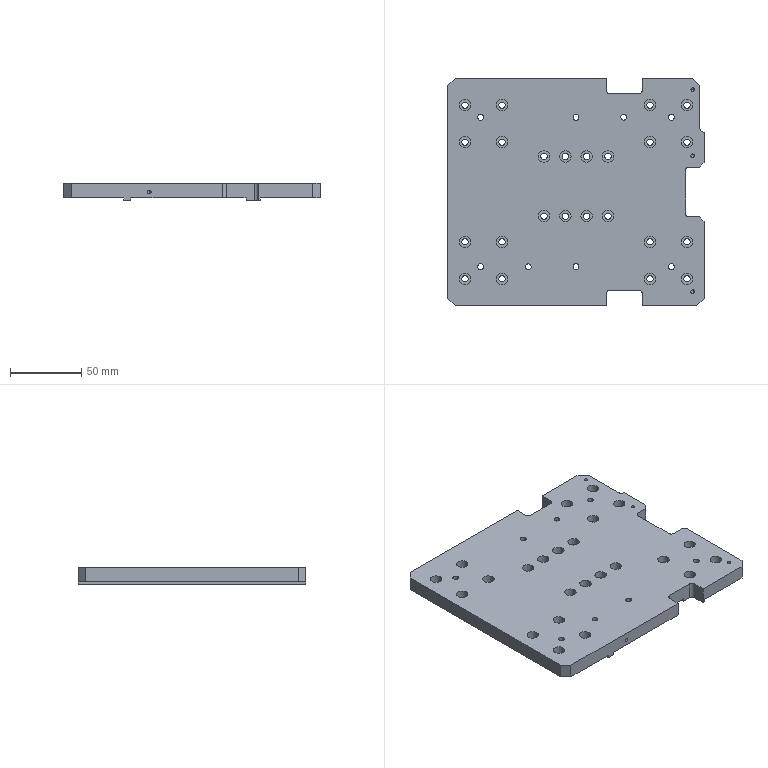Part | NX | features BREP 1 | 1 solid | 224 faces | box 180 x 160 x 12 mm | volume 236462 mm3 | cylinder 143 | plane 65 | cone 16 | commonest cylinder face diameters 4.5 x48 8 x48 2.5 x12 4.2 x12 10 x8 4 x6